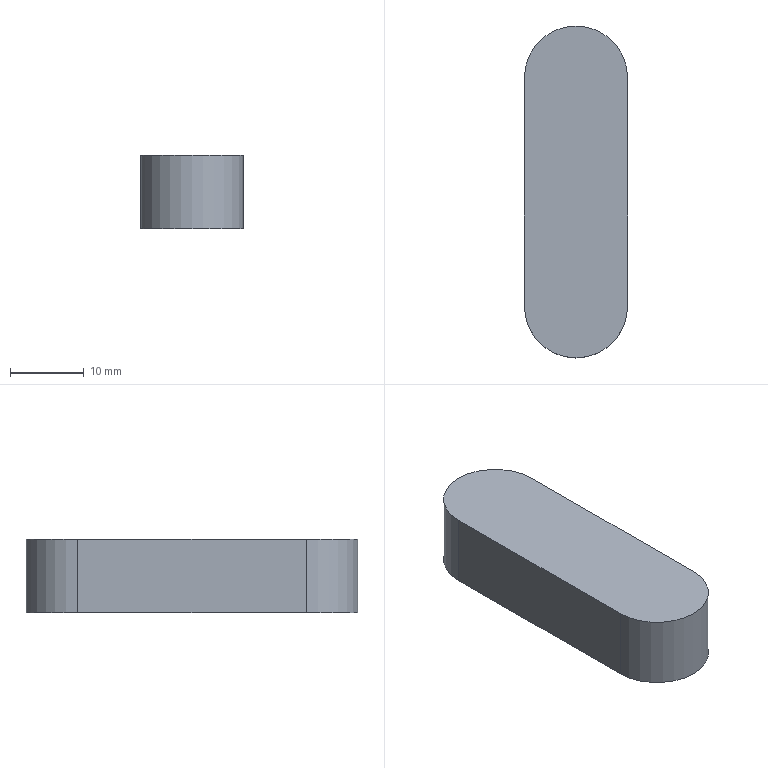Part | NX | 1 solid | 6 faces | box 14 x 45 x 10 mm | volume 5879 mm3 | plane 4 | cylinder 2 | commonest cylinder face diameters 14 x2
STEP:
#1=CARTESIAN_POINT('',(-7.,15.5,0.));
#2=VERTEX_POINT('',#1);
#3=CARTESIAN_POINT('',(-7.,-15.5,0.));
#4=VERTEX_POINT('',#3);
#5=CARTESIAN_POINT('',(-7.,22.5,0.));
#6=DIRECTION('',(0.,-1.,0.));
#7=VECTOR('',#6,1.);
#8=LINE('',#5,#7);
#9=EDGE_CURVE('',#2,#4,#8,.T.);
#10=ORIENTED_EDGE('',*,*,#9,.T.);
#11=CARTESIAN_POINT('',(-7.,-15.5,10.));
#12=VERTEX_POINT('',#11);
#13=CARTESIAN_POINT('',(-7.,-15.5,10.));
#14=DIRECTION('',(0.,0.,1.));
#15=VECTOR('',#14,1.);
#16=LINE('',#13,#15);
#17=EDGE_CURVE('',#4,#12,#16,.T.);
#18=ORIENTED_EDGE('',*,*,#17,.T.);
#19=CARTESIAN_POINT('',(-7.,15.5,10.));
#20=VERTEX_POINT('',#19);
#21=CARTESIAN_POINT('',(-7.,22.5,10.));
#22=DIRECTION('',(0.,-1.,0.));
#23=VECTOR('',#22,1.);
#24=LINE('',#21,#23);
#25=EDGE_CURVE('',#20,#12,#24,.T.);
#26=ORIENTED_EDGE('',*,*,#25,.F.);
#27=CARTESIAN_POINT('',(-7.,15.5,10.));
#28=DIRECTION('',(0.,0.,-1.));
#29=VECTOR('',#28,1.);
#30=LINE('',#27,#29);
#31=EDGE_CURVE('',#20,#2,#30,.T.);
#32=ORIENTED_EDGE('',*,*,#31,.T.);
#33=EDGE_LOOP('',(#10,#18,#26,#32));
#34=FACE_OUTER_BOUND('',#33,.T.);
#35=CARTESIAN_POINT('',(-7.,22.5,10.));
#36=DIRECTION('',(1.,0.,0.));
#37=DIRECTION('',(0.,-1.,0.));
#38=AXIS2_PLACEMENT_3D('',#35,#36,#37);
#39=PLANE('',#38);
#40=ADVANCED_FACE('',(#34),#39,.F.);
#41=CARTESIAN_POINT('',(7.,-15.5,10.));
#42=VERTEX_POINT('',#41);
#43=CARTESIAN_POINT('',(7.,15.5,10.));
#44=VERTEX_POINT('',#43);
#45=CARTESIAN_POINT('',(7.,-22.5,10.));
#46=DIRECTION('',(0.,1.,0.));
#47=VECTOR('',#46,1.);
#48=LINE('',#45,#47);
#49=EDGE_CURVE('',#42,#44,#48,.T.);
#50=ORIENTED_EDGE('',*,*,#49,.F.);
#51=CARTESIAN_POINT('',(7.,-15.5,0.));
#52=VERTEX_POINT('',#51);
#53=CARTESIAN_POINT('',(7.,-15.5,10.));
#54=DIRECTION('',(0.,0.,-1.));
#55=VECTOR('',#54,1.);
#56=LINE('',#53,#55);
#57=EDGE_CURVE('',#42,#52,#56,.T.);
#58=ORIENTED_EDGE('',*,*,#57,.T.);
#59=CARTESIAN_POINT('',(7.,15.5,0.));
#60=VERTEX_POINT('',#59);
#61=CARTESIAN_POINT('',(7.,-22.5,0.));
#62=DIRECTION('',(0.,1.,0.));
#63=VECTOR('',#62,1.);
#64=LINE('',#61,#63);
#65=EDGE_CURVE('',#52,#60,#64,.T.);
#66=ORIENTED_EDGE('',*,*,#65,.T.);
#67=CARTESIAN_POINT('',(7.,15.5,10.));
#68=DIRECTION('',(0.,0.,1.));
#69=VECTOR('',#68,1.);
#70=LINE('',#67,#69);
#71=EDGE_CURVE('',#60,#44,#70,.T.);
#72=ORIENTED_EDGE('',*,*,#71,.T.);
#73=EDGE_LOOP('',(#50,#58,#66,#72));
#74=FACE_OUTER_BOUND('',#73,.T.);
#75=CARTESIAN_POINT('',(7.,-22.5,10.));
#76=DIRECTION('',(-1.,0.,0.));
#77=DIRECTION('',(0.,1.,0.));
#78=AXIS2_PLACEMENT_3D('',#75,#76,#77);
#79=PLANE('',#78);
#80=ADVANCED_FACE('',(#74),#79,.F.);
#81=CARTESIAN_POINT('',(0.,-15.5,10.));
#82=DIRECTION('',(0.,0.,1.));
#83=DIRECTION('',(1.,0.,0.));
#84=AXIS2_PLACEMENT_3D('',#81,#82,#83);
#85=CIRCLE('',#84,7.);
#86=EDGE_CURVE('',#12,#42,#85,.T.);
#87=ORIENTED_EDGE('',*,*,#86,.T.);
#88=ORIENTED_EDGE('',*,*,#49,.T.);
#89=CARTESIAN_POINT('',(0.,15.5,10.));
#90=DIRECTION('',(0.,0.,1.));
#91=DIRECTION('',(1.,0.,0.));
#92=AXIS2_PLACEMENT_3D('',#89,#90,#91);
#93=CIRCLE('',#92,7.);
#94=EDGE_CURVE('',#44,#20,#93,.T.);
#95=ORIENTED_EDGE('',*,*,#94,.T.);
#96=ORIENTED_EDGE('',*,*,#25,.T.);
#97=EDGE_LOOP('',(#87,#88,#95,#96));
#98=FACE_OUTER_BOUND('',#97,.T.);
#99=CARTESIAN_POINT('',(0.,0.,10.));
#100=DIRECTION('',(0.,0.,1.));
#101=DIRECTION('',(-1.,0.,0.));
#102=AXIS2_PLACEMENT_3D('',#99,#100,#101);
#103=PLANE('',#102);
#104=ADVANCED_FACE('',(#98),#103,.T.);
#105=ORIENTED_EDGE('',*,*,#65,.F.);
#106=CARTESIAN_POINT('',(0.,-15.5,0.));
#107=DIRECTION('',(0.,0.,-1.));
#108=DIRECTION('',(1.,0.,0.));
#109=AXIS2_PLACEMENT_3D('',#106,#107,#108);
#110=CIRCLE('',#109,7.);
#111=EDGE_CURVE('',#52,#4,#110,.T.);
#112=ORIENTED_EDGE('',*,*,#111,.T.);
#113=ORIENTED_EDGE('',*,*,#9,.F.);
#114=CARTESIAN_POINT('',(0.,15.5,0.));
#115=DIRECTION('',(0.,0.,-1.));
#116=DIRECTION('',(1.,0.,0.));
#117=AXIS2_PLACEMENT_3D('',#114,#115,#116);
#118=CIRCLE('',#117,7.);
#119=EDGE_CURVE('',#2,#60,#118,.T.);
#120=ORIENTED_EDGE('',*,*,#119,.T.);
#121=EDGE_LOOP('',(#105,#112,#113,#120));
#122=FACE_OUTER_BOUND('',#121,.T.);
#123=CARTESIAN_POINT('',(0.,0.,0.));
#124=DIRECTION('',(0.,0.,1.));
#125=DIRECTION('',(-1.,0.,0.));
#126=AXIS2_PLACEMENT_3D('',#123,#124,#125);
#127=PLANE('',#126);
#128=ADVANCED_FACE('',(#122),#127,.F.);
#129=ORIENTED_EDGE('',*,*,#111,.F.);
#130=ORIENTED_EDGE('',*,*,#57,.F.);
#131=ORIENTED_EDGE('',*,*,#86,.F.);
#132=ORIENTED_EDGE('',*,*,#17,.F.);
#133=EDGE_LOOP('',(#129,#130,#131,#132));
#134=FACE_OUTER_BOUND('',#133,.T.);
#135=CARTESIAN_POINT('',(0.,-15.5,10.));
#136=DIRECTION('',(0.,0.,-1.));
#137=DIRECTION('',(1.,0.,0.));
#138=AXIS2_PLACEMENT_3D('',#135,#136,#137);
#139=CYLINDRICAL_SURFACE('',#138,7.);
#140=ADVANCED_FACE('',(#134),#139,.T.);
#141=ORIENTED_EDGE('',*,*,#31,.F.);
#142=ORIENTED_EDGE('',*,*,#94,.F.);
#143=ORIENTED_EDGE('',*,*,#71,.F.);
#144=ORIENTED_EDGE('',*,*,#119,.F.);
#145=EDGE_LOOP('',(#141,#142,#143,#144));
#146=FACE_OUTER_BOUND('',#145,.T.);
#147=CARTESIAN_POINT('',(0.,15.5,10.));
#148=DIRECTION('',(0.,0.,-1.));
#149=DIRECTION('',(1.,0.,0.));
#150=AXIS2_PLACEMENT_3D('',#147,#148,#149);
#151=CYLINDRICAL_SURFACE('',#150,7.);
#152=ADVANCED_FACE('',(#146),#151,.T.);
#153=CLOSED_SHELL('',(#40,#80,#104,#128,#140,#152));
#154=MANIFOLD_SOLID_BREP('',#153);
#155=(LENGTH_UNIT()NAMED_UNIT(*)SI_UNIT(.MILLI.,.METRE.));
#156=UNCERTAINTY_MEASURE_WITH_UNIT(LENGTH_MEASURE(0.00002),#155,'','');
#157=(NAMED_UNIT(*)PLANE_ANGLE_UNIT()SI_UNIT($,.RADIAN.));
#158=PLANE_ANGLE_MEASURE_WITH_UNIT(PLANE_ANGLE_MEASURE(0.01745),#157);
#159=DIMENSIONAL_EXPONENTS(0.,0.,0.,0.,0.,0.,0.);
#160=(CONVERSION_BASED_UNIT('DEGREE',#158)NAMED_UNIT(#159)PLANE_ANGLE_UNIT());
#161=(NAMED_UNIT(*)SI_UNIT($,.STERADIAN.)SOLID_ANGLE_UNIT());
#162=(GEOMETRIC_REPRESENTATION_CONTEXT(3)GLOBAL_UNCERTAINTY_ASSIGNED_CONTEXT((#156))GLOBAL_UNIT_ASSIGNED_CONTEXT((#155,#160,#161))REPRESENTATION_CONTEXT('',''));
#163=ADVANCED_BREP_SHAPE_REPRESENTATION('',(#154),#162);